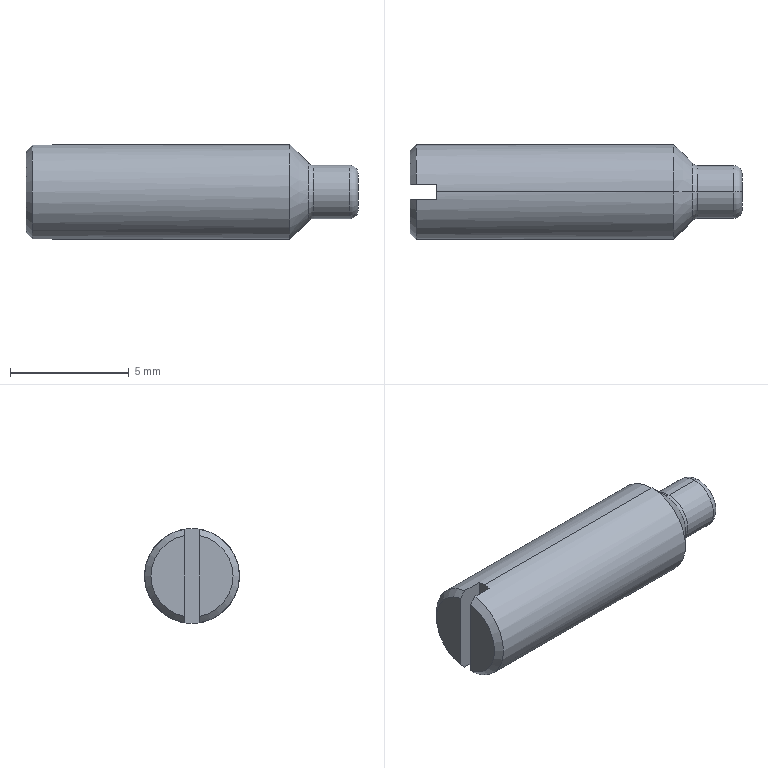Part | SolidWorks | features Cut 1, Fillet 1, Revolution 1 | 1 solid | 18 faces | box 14 x 4 x 4 mm | volume 151.43 mm3 | plane 6 | torus 4 | cylinder 4 | cone 4 | commonest cylinder face diameters 2.25 x2 4 x2
STEP:
#1=CARTESIAN_POINT('',(11.901,0.,-1.224));
#2=VERTEX_POINT('',#1);
#3=CARTESIAN_POINT('',(11.901,0.,1.224));
#4=VERTEX_POINT('',#3);
#5=CARTESIAN_POINT('',(11.901,0.,0.));
#6=DIRECTION('',(-1.,0.,0.));
#7=DIRECTION('',(0.,0.,1.));
#8=AXIS2_PLACEMENT_3D('',#5,#6,#7);
#9=CIRCLE('',#8,1.224);
#10=EDGE_CURVE('',#2,#4,#9,.T.);
#11=ORIENTED_EDGE('',*,*,#10,.F.);
#12=CARTESIAN_POINT('',(12.14,0.,-1.125));
#13=VERTEX_POINT('',#12);
#14=CARTESIAN_POINT('',(12.14,0.,-1.462));
#15=DIRECTION('',(0.,1.,0.));
#16=DIRECTION('',(0.,0.,1.));
#17=AXIS2_PLACEMENT_3D('',#14,#15,#16);
#18=CIRCLE('',#17,0.3375);
#19=EDGE_CURVE('',#2,#13,#18,.T.);
#20=ORIENTED_EDGE('',*,*,#19,.T.);
#21=CARTESIAN_POINT('',(12.14,0.,1.125));
#22=VERTEX_POINT('',#21);
#23=CARTESIAN_POINT('',(12.14,0.,0.));
#24=DIRECTION('',(1.,0.,0.));
#25=DIRECTION('',(0.,0.,1.));
#26=AXIS2_PLACEMENT_3D('',#23,#24,#25);
#27=CIRCLE('',#26,1.125);
#28=EDGE_CURVE('',#22,#13,#27,.T.);
#29=ORIENTED_EDGE('',*,*,#28,.F.);
#30=CARTESIAN_POINT('',(12.14,0.,1.462));
#31=DIRECTION('',(0.,-1.,0.));
#32=DIRECTION('',(0.,0.,-1.));
#33=AXIS2_PLACEMENT_3D('',#30,#31,#32);
#34=CIRCLE('',#33,0.3375);
#35=EDGE_CURVE('',#4,#22,#34,.T.);
#36=ORIENTED_EDGE('',*,*,#35,.F.);
#37=EDGE_LOOP('',(#11,#20,#29,#36));
#38=FACE_OUTER_BOUND('',#37,.T.);
#39=CARTESIAN_POINT('',(12.14,0.,0.));
#40=DIRECTION('',(-1.,0.,0.));
#41=DIRECTION('',(0.,0.,1.));
#42=AXIS2_PLACEMENT_3D('',#39,#40,#41);
#43=TOROIDAL_SURFACE('',#42,1.462,0.3375);
#44=ADVANCED_FACE('',(#38),#43,.F.);
#45=CARTESIAN_POINT('',(14.,0.,-0.7875));
#46=VERTEX_POINT('',#45);
#47=CARTESIAN_POINT('',(14.,0.,0.7875));
#48=VERTEX_POINT('',#47);
#49=CARTESIAN_POINT('',(14.,0.,0.));
#50=DIRECTION('',(1.,0.,0.));
#51=DIRECTION('',(0.,0.,1.));
#52=AXIS2_PLACEMENT_3D('',#49,#50,#51);
#53=CIRCLE('',#52,0.7875);
#54=EDGE_CURVE('',#46,#48,#53,.T.);
#55=ORIENTED_EDGE('',*,*,#54,.F.);
#56=CARTESIAN_POINT('',(13.663,0.,-1.125));
#57=VERTEX_POINT('',#56);
#58=CARTESIAN_POINT('',(13.663,0.,-0.7875));
#59=DIRECTION('',(0.,1.,0.));
#60=DIRECTION('',(0.,0.,1.));
#61=AXIS2_PLACEMENT_3D('',#58,#59,#60);
#62=CIRCLE('',#61,0.3375);
#63=EDGE_CURVE('',#46,#57,#62,.T.);
#64=ORIENTED_EDGE('',*,*,#63,.T.);
#65=CARTESIAN_POINT('',(13.663,0.,1.125));
#66=VERTEX_POINT('',#65);
#67=CARTESIAN_POINT('',(13.663,0.,0.));
#68=DIRECTION('',(-1.,0.,0.));
#69=DIRECTION('',(0.,0.,1.));
#70=AXIS2_PLACEMENT_3D('',#67,#68,#69);
#71=CIRCLE('',#70,1.125);
#72=EDGE_CURVE('',#66,#57,#71,.T.);
#73=ORIENTED_EDGE('',*,*,#72,.F.);
#74=CARTESIAN_POINT('',(13.663,0.,0.7875));
#75=DIRECTION('',(0.,-1.,0.));
#76=DIRECTION('',(0.,0.,-1.));
#77=AXIS2_PLACEMENT_3D('',#74,#75,#76);
#78=CIRCLE('',#77,0.3375);
#79=EDGE_CURVE('',#48,#66,#78,.T.);
#80=ORIENTED_EDGE('',*,*,#79,.F.);
#81=EDGE_LOOP('',(#55,#64,#73,#80));
#82=FACE_OUTER_BOUND('',#81,.T.);
#83=CARTESIAN_POINT('',(13.663,0.,0.));
#84=DIRECTION('',(-1.,0.,0.));
#85=DIRECTION('',(0.,0.,1.));
#86=AXIS2_PLACEMENT_3D('',#83,#84,#85);
#87=TOROIDAL_SURFACE('',#86,0.7875,0.3375);
#88=ADVANCED_FACE('',(#82),#87,.T.);
#89=ORIENTED_EDGE('',*,*,#72,.T.);
#90=CARTESIAN_POINT('',(-1.425,0.,-1.125));
#91=DIRECTION('',(-1.,0.,0.));
#92=VECTOR('',#91,1000.);
#93=LINE('',#90,#92);
#94=EDGE_CURVE('',#57,#13,#93,.T.);
#95=ORIENTED_EDGE('',*,*,#94,.T.);
#96=CARTESIAN_POINT('',(12.14,0.,0.));
#97=DIRECTION('',(1.,0.,0.));
#98=DIRECTION('',(0.,0.,1.));
#99=AXIS2_PLACEMENT_3D('',#96,#97,#98);
#100=CIRCLE('',#99,1.125);
#101=EDGE_CURVE('',#13,#22,#100,.T.);
#102=ORIENTED_EDGE('',*,*,#101,.T.);
#103=CARTESIAN_POINT('',(-1.425,0.,1.125));
#104=DIRECTION('',(-1.,0.,0.));
#105=VECTOR('',#104,1000.);
#106=LINE('',#103,#105);
#107=EDGE_CURVE('',#66,#22,#106,.T.);
#108=ORIENTED_EDGE('',*,*,#107,.F.);
#109=EDGE_LOOP('',(#89,#95,#102,#108));
#110=FACE_OUTER_BOUND('',#109,.T.);
#111=CARTESIAN_POINT('',(-1.425,0.,0.));
#112=DIRECTION('',(-1.,0.,0.));
#113=DIRECTION('',(0.,0.,1.));
#114=AXIS2_PLACEMENT_3D('',#111,#112,#113);
#115=CYLINDRICAL_SURFACE('',#114,1.125);
#116=ADVANCED_FACE('',(#110),#115,.T.);
#117=CARTESIAN_POINT('',(11.901,0.,0.));
#118=DIRECTION('',(-1.,0.,0.));
#119=DIRECTION('',(0.,0.,1.));
#120=AXIS2_PLACEMENT_3D('',#117,#118,#119);
#121=CIRCLE('',#120,1.224);
#122=EDGE_CURVE('',#4,#2,#121,.T.);
#123=ORIENTED_EDGE('',*,*,#122,.T.);
#124=CARTESIAN_POINT('',(11.125,0.,-2.));
#125=VERTEX_POINT('',#124);
#126=CARTESIAN_POINT('',(12.,0.,-1.125));
#127=DIRECTION('',(-0.7071,0.,-0.7071));
#128=VECTOR('',#127,1000.);
#129=LINE('',#126,#128);
#130=EDGE_CURVE('',#2,#125,#129,.T.);
#131=ORIENTED_EDGE('',*,*,#130,.T.);
#132=CARTESIAN_POINT('',(11.125,0.,2.));
#133=VERTEX_POINT('',#132);
#134=CARTESIAN_POINT('',(11.125,0.,0.));
#135=DIRECTION('',(-1.,0.,0.));
#136=DIRECTION('',(0.,0.,1.));
#137=AXIS2_PLACEMENT_3D('',#134,#135,#136);
#138=CIRCLE('',#137,2.);
#139=EDGE_CURVE('',#133,#125,#138,.T.);
#140=ORIENTED_EDGE('',*,*,#139,.F.);
#141=CARTESIAN_POINT('',(12.,0.,1.125));
#142=DIRECTION('',(-0.7071,0.,0.7071));
#143=VECTOR('',#142,1000.);
#144=LINE('',#141,#143);
#145=EDGE_CURVE('',#4,#133,#144,.T.);
#146=ORIENTED_EDGE('',*,*,#145,.F.);
#147=EDGE_LOOP('',(#123,#131,#140,#146));
#148=FACE_OUTER_BOUND('',#147,.T.);
#149=CARTESIAN_POINT('',(12.,0.,0.));
#150=DIRECTION('',(-1.,0.,0.));
#151=DIRECTION('',(0.,0.,1.));
#152=AXIS2_PLACEMENT_3D('',#149,#150,#151);
#153=CONICAL_SURFACE('',#152,1.125,0.7854);
#154=ADVANCED_FACE('',(#148),#153,.T.);
#155=ORIENTED_EDGE('',*,*,#139,.T.);
#156=CARTESIAN_POINT('',(1.12,0.,-2.));
#157=VERTEX_POINT('',#156);
#158=CARTESIAN_POINT('',(-1.425,0.,-2.));
#159=DIRECTION('',(-1.,0.,0.));
#160=VECTOR('',#159,1000.);
#161=LINE('',#158,#160);
#162=EDGE_CURVE('',#125,#157,#161,.T.);
#163=ORIENTED_EDGE('',*,*,#162,.T.);
#164=CARTESIAN_POINT('',(1.12,0.3,-1.977));
#165=VERTEX_POINT('',#164);
#166=CARTESIAN_POINT('',(1.12,0.,0.));
#167=DIRECTION('',(1.,0.,0.));
#168=DIRECTION('',(0.,0.,-1.));
#169=AXIS2_PLACEMENT_3D('',#166,#167,#168);
#170=CIRCLE('',#169,2.);
#171=EDGE_CURVE('',#157,#165,#170,.T.);
#172=ORIENTED_EDGE('',*,*,#171,.T.);
#173=CARTESIAN_POINT('',(0.268,0.3,-1.977));
#174=VERTEX_POINT('',#173);
#175=CARTESIAN_POINT('',(-1.425,0.3,-1.977));
#176=DIRECTION('',(-1.,0.,0.));
#177=VECTOR('',#176,1000.);
#178=LINE('',#175,#177);
#179=EDGE_CURVE('',#165,#174,#178,.T.);
#180=ORIENTED_EDGE('',*,*,#179,.T.);
#181=CARTESIAN_POINT('',(0.268,0.3,1.977));
#182=VERTEX_POINT('',#181);
#183=CARTESIAN_POINT('',(0.268,0.,0.));
#184=DIRECTION('',(-1.,0.,0.));
#185=DIRECTION('',(0.,0.,1.));
#186=AXIS2_PLACEMENT_3D('',#183,#184,#185);
#187=CIRCLE('',#186,2.);
#188=EDGE_CURVE('',#182,#174,#187,.T.);
#189=ORIENTED_EDGE('',*,*,#188,.F.);
#190=CARTESIAN_POINT('',(1.12,0.3,1.977));
#191=VERTEX_POINT('',#190);
#192=CARTESIAN_POINT('',(-1.425,0.3,1.977));
#193=DIRECTION('',(1.,0.,0.));
#194=VECTOR('',#193,1000.);
#195=LINE('',#192,#194);
#196=EDGE_CURVE('',#182,#191,#195,.T.);
#197=ORIENTED_EDGE('',*,*,#196,.T.);
#198=CARTESIAN_POINT('',(1.12,0.,2.));
#199=VERTEX_POINT('',#198);
#200=CARTESIAN_POINT('',(1.12,0.,0.));
#201=DIRECTION('',(1.,0.,0.));
#202=DIRECTION('',(0.,0.,-1.));
#203=AXIS2_PLACEMENT_3D('',#200,#201,#202);
#204=CIRCLE('',#203,2.);
#205=EDGE_CURVE('',#191,#199,#204,.T.);
#206=ORIENTED_EDGE('',*,*,#205,.T.);
#207=CARTESIAN_POINT('',(-1.425,0.,2.));
#208=DIRECTION('',(-1.,0.,0.));
#209=VECTOR('',#208,1000.);
#210=LINE('',#207,#209);
#211=EDGE_CURVE('',#133,#199,#210,.T.);
#212=ORIENTED_EDGE('',*,*,#211,.F.);
#213=EDGE_LOOP('',(#155,#163,#172,#180,#189,#197,#206,#212));
#214=FACE_OUTER_BOUND('',#213,.T.);
#215=CARTESIAN_POINT('',(-1.425,0.,0.));
#216=DIRECTION('',(-1.,0.,0.));
#217=DIRECTION('',(0.,0.,1.));
#218=AXIS2_PLACEMENT_3D('',#215,#216,#217);
#219=CYLINDRICAL_SURFACE('',#218,2.);
#220=ADVANCED_FACE('',(#214),#219,.T.);
#221=CARTESIAN_POINT('',(0.,0.3,1.706));
#222=VERTEX_POINT('',#221);
#223=CARTESIAN_POINT('',(0.,0.3,-1.706));
#224=VERTEX_POINT('',#223);
#225=CARTESIAN_POINT('',(0.,0.,0.));
#226=DIRECTION('',(-1.,0.,0.));
#227=DIRECTION('',(0.,0.,1.));
#228=AXIS2_PLACEMENT_3D('',#225,#226,#227);
#229=CIRCLE('',#228,1.732);
#230=EDGE_CURVE('',#222,#224,#229,.T.);
#231=ORIENTED_EDGE('',*,*,#230,.T.);
#232=CARTESIAN_POINT('',(0.,0.3,-50.));
#233=DIRECTION('',(0.,0.,1.));
#234=VECTOR('',#233,1000.);
#235=LINE('',#232,#234);
#236=EDGE_CURVE('',#224,#222,#235,.T.);
#237=ORIENTED_EDGE('',*,*,#236,.T.);
#238=EDGE_LOOP('',(#231,#237));
#239=FACE_OUTER_BOUND('',#238,.T.);
#240=CARTESIAN_POINT('',(0.,0.,0.));
#241=DIRECTION('',(1.,0.,0.));
#242=DIRECTION('',(0.,0.,-1.));
#243=AXIS2_PLACEMENT_3D('',#240,#241,#242);
#244=PLANE('',#243);
#245=ADVANCED_FACE('',(#239),#244,.F.);
#246=ORIENTED_EDGE('',*,*,#188,.T.);
#247=CARTESIAN_POINT('',(0.268,0.3,-1.977));
#248=CARTESIAN_POINT('',(0.1786,0.3,-1.887));
#249=CARTESIAN_POINT('',(0.08924,0.3,-1.796));
#250=CARTESIAN_POINT('',(0.,0.3,-1.706));
#251=B_SPLINE_CURVE_WITH_KNOTS('',3,(#247,#248,#249,#250),.UNSPECIFIED.,.F.,.F.,(4,4),(0.003411,0.003792),.UNSPECIFIED.);
#252=EDGE_CURVE('',#174,#224,#251,.T.);
#253=ORIENTED_EDGE('',*,*,#252,.T.);
#254=ORIENTED_EDGE('',*,*,#230,.F.);
#255=CARTESIAN_POINT('',(0.,0.3,1.706));
#256=CARTESIAN_POINT('',(0.08924,0.3,1.796));
#257=CARTESIAN_POINT('',(0.1786,0.3,1.887));
#258=CARTESIAN_POINT('',(0.268,0.3,1.977));
#259=B_SPLINE_CURVE_WITH_KNOTS('',3,(#255,#256,#257,#258),.UNSPECIFIED.,.F.,.F.,(4,4),(0.008312,0.008697),.UNSPECIFIED.);
#260=EDGE_CURVE('',#222,#182,#259,.T.);
#261=ORIENTED_EDGE('',*,*,#260,.T.);
#262=EDGE_LOOP('',(#246,#253,#254,#261));
#263=FACE_OUTER_BOUND('',#262,.T.);
#264=CARTESIAN_POINT('',(0.268,0.,0.));
#265=DIRECTION('',(1.,0.,0.));
#266=DIRECTION('',(0.,0.,-1.));
#267=AXIS2_PLACEMENT_3D('',#264,#265,#266);
#268=CONICAL_SURFACE('',#267,2.,0.7854);
#269=ADVANCED_FACE('',(#263),#268,.T.);
#270=CARTESIAN_POINT('',(0.,-0.3,-1.706));
#271=VERTEX_POINT('',#270);
#272=CARTESIAN_POINT('',(0.,-0.3,1.706));
#273=VERTEX_POINT('',#272);
#274=CARTESIAN_POINT('',(0.,0.,0.));
#275=DIRECTION('',(-1.,0.,0.));
#276=DIRECTION('',(0.,0.,1.));
#277=AXIS2_PLACEMENT_3D('',#274,#275,#276);
#278=CIRCLE('',#277,1.732);
#279=EDGE_CURVE('',#271,#273,#278,.T.);
#280=ORIENTED_EDGE('',*,*,#279,.T.);
#281=CARTESIAN_POINT('',(0.,-0.3,-50.));
#282=DIRECTION('',(0.,0.,1.));
#283=VECTOR('',#282,1000.);
#284=LINE('',#281,#283);
#285=EDGE_CURVE('',#271,#273,#284,.T.);
#286=ORIENTED_EDGE('',*,*,#285,.F.);
#287=EDGE_LOOP('',(#280,#286));
#288=FACE_OUTER_BOUND('',#287,.T.);
#289=CARTESIAN_POINT('',(0.,0.,0.));
#290=DIRECTION('',(1.,0.,0.));
#291=DIRECTION('',(0.,0.,-1.));
#292=AXIS2_PLACEMENT_3D('',#289,#290,#291);
#293=PLANE('',#292);
#294=ADVANCED_FACE('',(#288),#293,.F.);
#295=CARTESIAN_POINT('',(0.268,-0.3,-1.977));
#296=VERTEX_POINT('',#295);
#297=CARTESIAN_POINT('',(0.268,-0.3,1.977));
#298=VERTEX_POINT('',#297);
#299=CARTESIAN_POINT('',(0.268,0.,0.));
#300=DIRECTION('',(-1.,0.,0.));
#301=DIRECTION('',(0.,0.,1.));
#302=AXIS2_PLACEMENT_3D('',#299,#300,#301);
#303=CIRCLE('',#302,2.);
#304=EDGE_CURVE('',#296,#298,#303,.T.);
#305=ORIENTED_EDGE('',*,*,#304,.T.);
#306=CARTESIAN_POINT('',(0.268,-0.3,1.977));
#307=CARTESIAN_POINT('',(0.1786,-0.3,1.887));
#308=CARTESIAN_POINT('',(0.08924,-0.3,1.796));
#309=CARTESIAN_POINT('',(0.,-0.3,1.706));
#310=B_SPLINE_CURVE_WITH_KNOTS('',3,(#306,#307,#308,#309),.UNSPECIFIED.,.F.,.F.,(4,4),(0.003411,0.003792),.UNSPECIFIED.);
#311=EDGE_CURVE('',#298,#273,#310,.T.);
#312=ORIENTED_EDGE('',*,*,#311,.T.);
#313=ORIENTED_EDGE('',*,*,#279,.F.);
#314=CARTESIAN_POINT('',(0.,-0.3,-1.706));
#315=CARTESIAN_POINT('',(0.08924,-0.3,-1.796));
#316=CARTESIAN_POINT('',(0.1786,-0.3,-1.887));
#317=CARTESIAN_POINT('',(0.268,-0.3,-1.977));
#318=B_SPLINE_CURVE_WITH_KNOTS('',3,(#314,#315,#316,#317),.UNSPECIFIED.,.F.,.F.,(4,4),(0.008312,0.008697),.UNSPECIFIED.);
#319=EDGE_CURVE('',#271,#296,#318,.T.);
#320=ORIENTED_EDGE('',*,*,#319,.T.);
#321=EDGE_LOOP('',(#305,#312,#313,#320));
#322=FACE_OUTER_BOUND('',#321,.T.);
#323=CARTESIAN_POINT('',(0.268,0.,0.));
#324=DIRECTION('',(1.,0.,0.));
#325=DIRECTION('',(0.,0.,-1.));
#326=AXIS2_PLACEMENT_3D('',#323,#324,#325);
#327=CONICAL_SURFACE('',#326,2.,0.7854);
#328=ADVANCED_FACE('',(#322),#327,.T.);
#329=ORIENTED_EDGE('',*,*,#162,.F.);
#330=CARTESIAN_POINT('',(11.125,0.,0.));
#331=DIRECTION('',(-1.,0.,0.));
#332=DIRECTION('',(0.,0.,1.));
#333=AXIS2_PLACEMENT_3D('',#330,#331,#332);
#334=CIRCLE('',#333,2.);
#335=EDGE_CURVE('',#125,#133,#334,.T.);
#336=ORIENTED_EDGE('',*,*,#335,.T.);
#337=ORIENTED_EDGE('',*,*,#211,.T.);
#338=CARTESIAN_POINT('',(1.12,-0.3,1.977));
#339=VERTEX_POINT('',#338);
#340=CARTESIAN_POINT('',(1.12,0.,0.));
#341=DIRECTION('',(1.,0.,0.));
#342=DIRECTION('',(0.,0.,-1.));
#343=AXIS2_PLACEMENT_3D('',#340,#341,#342);
#344=CIRCLE('',#343,2.);
#345=EDGE_CURVE('',#199,#339,#344,.T.);
#346=ORIENTED_EDGE('',*,*,#345,.T.);
#347=CARTESIAN_POINT('',(-1.425,-0.3,1.977));
#348=DIRECTION('',(-1.,0.,0.));
#349=VECTOR('',#348,1000.);
#350=LINE('',#347,#349);
#351=EDGE_CURVE('',#339,#298,#350,.T.);
#352=ORIENTED_EDGE('',*,*,#351,.T.);
#353=ORIENTED_EDGE('',*,*,#304,.F.);
#354=CARTESIAN_POINT('',(1.12,-0.3,-1.977));
#355=VERTEX_POINT('',#354);
#356=CARTESIAN_POINT('',(-1.425,-0.3,-1.977));
#357=DIRECTION('',(1.,0.,0.));
#358=VECTOR('',#357,1000.);
#359=LINE('',#356,#358);
#360=EDGE_CURVE('',#296,#355,#359,.T.);
#361=ORIENTED_EDGE('',*,*,#360,.T.);
#362=CARTESIAN_POINT('',(1.12,0.,0.));
#363=DIRECTION('',(1.,0.,0.));
#364=DIRECTION('',(0.,0.,-1.));
#365=AXIS2_PLACEMENT_3D('',#362,#363,#364);
#366=CIRCLE('',#365,2.);
#367=EDGE_CURVE('',#355,#157,#366,.T.);
#368=ORIENTED_EDGE('',*,*,#367,.T.);
#369=EDGE_LOOP('',(#329,#336,#337,#346,#352,#353,#361,#368));
#370=FACE_OUTER_BOUND('',#369,.T.);
#371=CARTESIAN_POINT('',(-1.425,0.,0.));
#372=DIRECTION('',(-1.,0.,0.));
#373=DIRECTION('',(0.,0.,1.));
#374=AXIS2_PLACEMENT_3D('',#371,#372,#373);
#375=CYLINDRICAL_SURFACE('',#374,2.);
#376=ADVANCED_FACE('',(#370),#375,.T.);
#377=ORIENTED_EDGE('',*,*,#130,.F.);
#378=ORIENTED_EDGE('',*,*,#10,.T.);
#379=ORIENTED_EDGE('',*,*,#145,.T.);
#380=ORIENTED_EDGE('',*,*,#335,.F.);
#381=EDGE_LOOP('',(#377,#378,#379,#380));
#382=FACE_OUTER_BOUND('',#381,.T.);
#383=CARTESIAN_POINT('',(12.,0.,0.));
#384=DIRECTION('',(-1.,0.,0.));
#385=DIRECTION('',(0.,0.,1.));
#386=AXIS2_PLACEMENT_3D('',#383,#384,#385);
#387=CONICAL_SURFACE('',#386,1.125,0.7854);
#388=ADVANCED_FACE('',(#382),#387,.T.);
#389=ORIENTED_EDGE('',*,*,#94,.F.);
#390=CARTESIAN_POINT('',(13.663,0.,0.));
#391=DIRECTION('',(-1.,0.,0.));
#392=DIRECTION('',(0.,0.,1.));
#393=AXIS2_PLACEMENT_3D('',#390,#391,#392);
#394=CIRCLE('',#393,1.125);
#395=EDGE_CURVE('',#57,#66,#394,.T.);
#396=ORIENTED_EDGE('',*,*,#395,.T.);
#397=ORIENTED_EDGE('',*,*,#107,.T.);
#398=ORIENTED_EDGE('',*,*,#28,.T.);
#399=EDGE_LOOP('',(#389,#396,#397,#398));
#400=FACE_OUTER_BOUND('',#399,.T.);
#401=CARTESIAN_POINT('',(-1.425,0.,0.));
#402=DIRECTION('',(-1.,0.,0.));
#403=DIRECTION('',(0.,0.,1.));
#404=AXIS2_PLACEMENT_3D('',#401,#402,#403);
#405=CYLINDRICAL_SURFACE('',#404,1.125);
#406=ADVANCED_FACE('',(#400),#405,.T.);
#407=CARTESIAN_POINT('',(14.,0.,0.));
#408=DIRECTION('',(1.,0.,0.));
#409=DIRECTION('',(0.,0.,1.));
#410=AXIS2_PLACEMENT_3D('',#407,#408,#409);
#411=CIRCLE('',#410,0.7875);
#412=EDGE_CURVE('',#48,#46,#411,.T.);
#413=ORIENTED_EDGE('',*,*,#412,.T.);
#414=ORIENTED_EDGE('',*,*,#54,.T.);
#415=EDGE_LOOP('',(#413,#414));
#416=FACE_OUTER_BOUND('',#415,.T.);
#417=CARTESIAN_POINT('',(14.,1.125,0.));
#418=DIRECTION('',(-1.,0.,0.));
#419=DIRECTION('',(0.,0.,1.));
#420=AXIS2_PLACEMENT_3D('',#417,#418,#419);
#421=PLANE('',#420);
#422=ADVANCED_FACE('',(#416),#421,.F.);
#423=ORIENTED_EDGE('',*,*,#179,.F.);
#424=CARTESIAN_POINT('',(1.12,0.3,-50.));
#425=DIRECTION('',(0.,0.,1.));
#426=VECTOR('',#425,1000.);
#427=LINE('',#424,#426);
#428=EDGE_CURVE('',#165,#191,#427,.T.);
#429=ORIENTED_EDGE('',*,*,#428,.T.);
#430=ORIENTED_EDGE('',*,*,#196,.F.);
#431=ORIENTED_EDGE('',*,*,#260,.F.);
#432=ORIENTED_EDGE('',*,*,#236,.F.);
#433=ORIENTED_EDGE('',*,*,#252,.F.);
#434=EDGE_LOOP('',(#423,#429,#430,#431,#432,#433));
#435=FACE_OUTER_BOUND('',#434,.T.);
#436=CARTESIAN_POINT('',(0.,0.3,-50.));
#437=DIRECTION('',(0.,1.,0.));
#438=DIRECTION('',(0.,0.,1.));
#439=AXIS2_PLACEMENT_3D('',#436,#437,#438);
#440=PLANE('',#439);
#441=ADVANCED_FACE('',(#435),#440,.F.);
#442=ORIENTED_EDGE('',*,*,#428,.F.);
#443=ORIENTED_EDGE('',*,*,#171,.F.);
#444=ORIENTED_EDGE('',*,*,#367,.F.);
#445=CARTESIAN_POINT('',(1.12,-0.3,-50.));
#446=DIRECTION('',(0.,0.,1.));
#447=VECTOR('',#446,1000.);
#448=LINE('',#445,#447);
#449=EDGE_CURVE('',#355,#339,#448,.T.);
#450=ORIENTED_EDGE('',*,*,#449,.T.);
#451=ORIENTED_EDGE('',*,*,#345,.F.);
#452=ORIENTED_EDGE('',*,*,#205,.F.);
#453=EDGE_LOOP('',(#442,#443,#444,#450,#451,#452));
#454=FACE_OUTER_BOUND('',#453,.T.);
#455=CARTESIAN_POINT('',(1.12,0.3,-50.));
#456=DIRECTION('',(1.,0.,0.));
#457=DIRECTION('',(0.,0.,-1.));
#458=AXIS2_PLACEMENT_3D('',#455,#456,#457);
#459=PLANE('',#458);
#460=ADVANCED_FACE('',(#454),#459,.F.);
#461=ORIENTED_EDGE('',*,*,#351,.F.);
#462=ORIENTED_EDGE('',*,*,#449,.F.);
#463=ORIENTED_EDGE('',*,*,#360,.F.);
#464=ORIENTED_EDGE('',*,*,#319,.F.);
#465=ORIENTED_EDGE('',*,*,#285,.T.);
#466=ORIENTED_EDGE('',*,*,#311,.F.);
#467=EDGE_LOOP('',(#461,#462,#463,#464,#465,#466));
#468=FACE_OUTER_BOUND('',#467,.T.);
#469=CARTESIAN_POINT('',(0.,-0.3,-50.));
#470=DIRECTION('',(0.,-1.,0.));
#471=DIRECTION('',(0.,0.,-1.));
#472=AXIS2_PLACEMENT_3D('',#469,#470,#471);
#473=PLANE('',#472);
#474=ADVANCED_FACE('',(#468),#473,.F.);
#475=ORIENTED_EDGE('',*,*,#63,.F.);
#476=ORIENTED_EDGE('',*,*,#412,.F.);
#477=ORIENTED_EDGE('',*,*,#79,.T.);
#478=ORIENTED_EDGE('',*,*,#395,.F.);
#479=EDGE_LOOP('',(#475,#476,#477,#478));
#480=FACE_OUTER_BOUND('',#479,.T.);
#481=CARTESIAN_POINT('',(13.663,0.,0.));
#482=DIRECTION('',(-1.,0.,0.));
#483=DIRECTION('',(0.,0.,1.));
#484=AXIS2_PLACEMENT_3D('',#481,#482,#483);
#485=TOROIDAL_SURFACE('',#484,0.7875,0.3375);
#486=ADVANCED_FACE('',(#480),#485,.T.);
#487=ORIENTED_EDGE('',*,*,#19,.F.);
#488=ORIENTED_EDGE('',*,*,#122,.F.);
#489=ORIENTED_EDGE('',*,*,#35,.T.);
#490=ORIENTED_EDGE('',*,*,#101,.F.);
#491=EDGE_LOOP('',(#487,#488,#489,#490));
#492=FACE_OUTER_BOUND('',#491,.T.);
#493=CARTESIAN_POINT('',(12.14,0.,0.));
#494=DIRECTION('',(-1.,0.,0.));
#495=DIRECTION('',(0.,0.,1.));
#496=AXIS2_PLACEMENT_3D('',#493,#494,#495);
#497=TOROIDAL_SURFACE('',#496,1.462,0.3375);
#498=ADVANCED_FACE('',(#492),#497,.F.);
#499=CLOSED_SHELL('',(#44,#88,#116,#154,#220,#245,#269,#294,#328,#376,#388,#406,#422,#441,#460,#474,#486,#498));
#500=MANIFOLD_SOLID_BREP('',#499);
#501=CARTESIAN_POINT('',(0.,0.,0.));
#502=DIRECTION('',(0.,0.,1.));
#503=DIRECTION('',(1.,0.,0.));
#504=AXIS2_PLACEMENT_3D('',#501,#502,#503);
#505=(LENGTH_UNIT()NAMED_UNIT(*)SI_UNIT(.MILLI.,.METRE.));
#506=UNCERTAINTY_MEASURE_WITH_UNIT(LENGTH_MEASURE(0.00001),#505,'','');
#507=(NAMED_UNIT(*)PLANE_ANGLE_UNIT()SI_UNIT($,.RADIAN.));
#508=(NAMED_UNIT(*)SI_UNIT($,.STERADIAN.)SOLID_ANGLE_UNIT());
#509=(GEOMETRIC_REPRESENTATION_CONTEXT(3)GLOBAL_UNCERTAINTY_ASSIGNED_CONTEXT((#506))GLOBAL_UNIT_ASSIGNED_CONTEXT((#505,#507,#508))REPRESENTATION_CONTEXT('',''));
#510=ADVANCED_BREP_SHAPE_REPRESENTATION('',(#500,#504),#509);